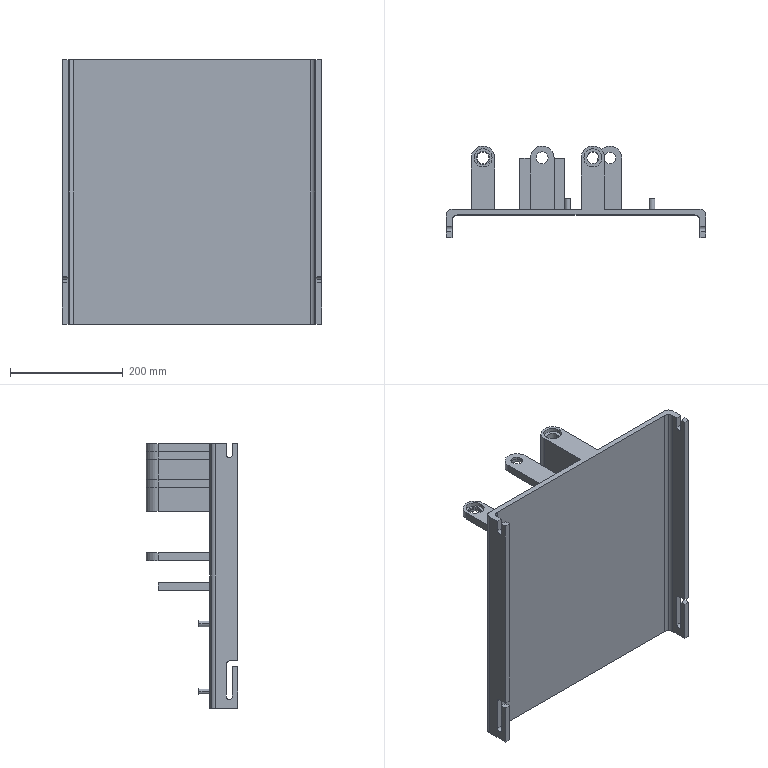Part | SolidWorks | features BaseBody 1 | 1 solid | 132 faces | box 460 x 162.384 x 469.5 mm | volume 3275559 mm3 | plane 63 | cylinder 61 | cone 8 | commonest cylinder face diameters 10 x14 32 x10 42 x9 20 x8 21 x8 5 x4